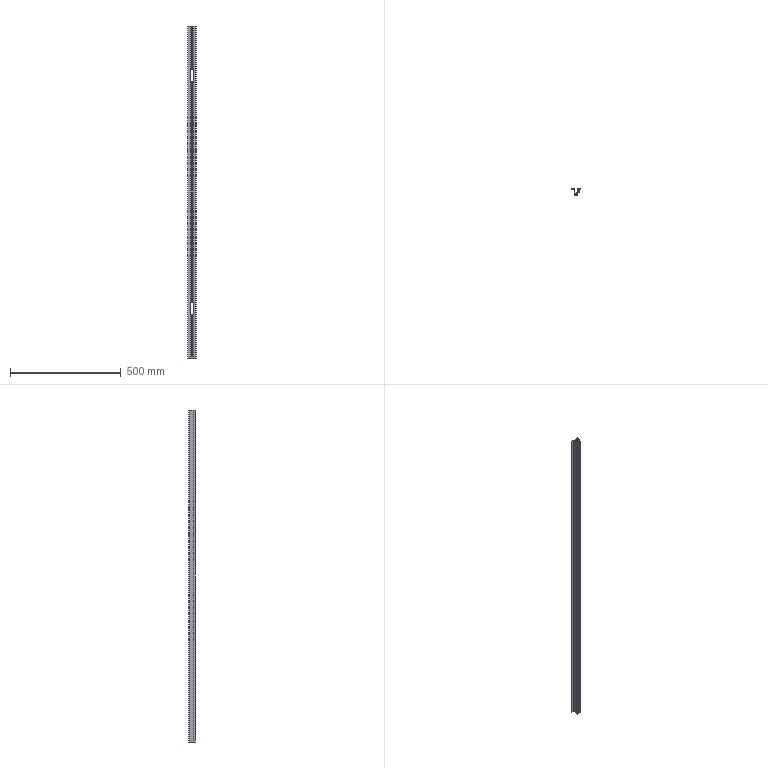Part | SolidWorks | features Cut 1, Extrusion 1, ICE 1 | 1 solid | 72 faces | box 40 x 29.5 x 1500 mm | volume 284523 mm3 | plane 51 | cylinder 21 | commonest cylinder face diameters 10 x14 2 x5 3 x2